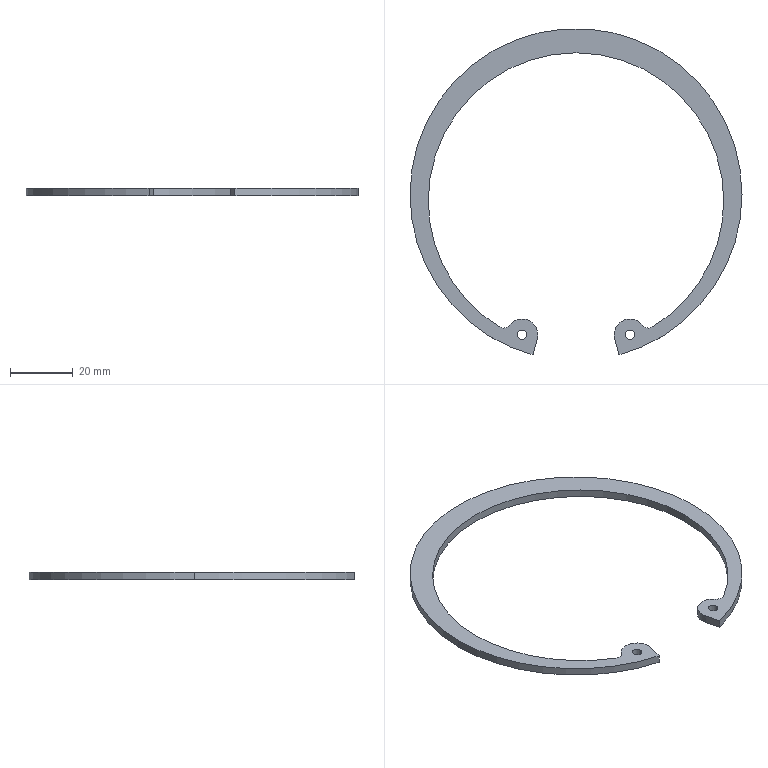Part | SolidWorks | features Extrusion 1 | 1 solid | 19 faces | box 105.5 x 103.703 x 2.5 mm | volume 4495 mm3 | cylinder 15 | plane 4 | commonest cylinder face diameters 3 x4 10 x3 93.9 x3 105.5 x3 5 x2
STEP:
#1=CARTESIAN_POINT('',(-18.607,-44.527,-2.5));
#2=VERTEX_POINT('',#1);
#3=CARTESIAN_POINT('',(-15.607,-44.527,-2.5));
#4=VERTEX_POINT('',#3);
#5=CARTESIAN_POINT('',(-17.107,-44.527,-2.5));
#6=DIRECTION('',(0.,0.,1.));
#7=DIRECTION('',(1.,0.,0.));
#8=AXIS2_PLACEMENT_3D('',#5,#6,#7);
#9=CIRCLE('',#8,1.5);
#10=EDGE_CURVE('',#2,#4,#9,.T.);
#11=ORIENTED_EDGE('',*,*,#10,.F.);
#12=CARTESIAN_POINT('',(-18.607,-44.527,0.));
#13=VERTEX_POINT('',#12);
#14=CARTESIAN_POINT('',(-18.607,-44.527,-2.5));
#15=DIRECTION('',(0.,0.,1.));
#16=VECTOR('',#15,1000.);
#17=LINE('',#14,#16);
#18=EDGE_CURVE('',#2,#13,#17,.T.);
#19=ORIENTED_EDGE('',*,*,#18,.T.);
#20=CARTESIAN_POINT('',(-15.607,-44.527,0.));
#21=VERTEX_POINT('',#20);
#22=CARTESIAN_POINT('',(-17.107,-44.527,0.));
#23=DIRECTION('',(0.,0.,1.));
#24=DIRECTION('',(1.,0.,0.));
#25=AXIS2_PLACEMENT_3D('',#22,#23,#24);
#26=CIRCLE('',#25,1.5);
#27=EDGE_CURVE('',#13,#21,#26,.T.);
#28=ORIENTED_EDGE('',*,*,#27,.T.);
#29=CARTESIAN_POINT('',(-15.607,-44.527,-2.5));
#30=DIRECTION('',(0.,0.,1.));
#31=VECTOR('',#30,1000.);
#32=LINE('',#29,#31);
#33=EDGE_CURVE('',#4,#21,#32,.T.);
#34=ORIENTED_EDGE('',*,*,#33,.F.);
#35=EDGE_LOOP('',(#11,#19,#28,#34));
#36=FACE_OUTER_BOUND('',#35,.T.);
#37=CARTESIAN_POINT('',(-17.107,-44.527,-2.5));
#38=DIRECTION('',(0.,0.,1.));
#39=DIRECTION('',(1.,0.,0.));
#40=AXIS2_PLACEMENT_3D('',#37,#38,#39);
#41=CYLINDRICAL_SURFACE('',#40,1.5);
#42=ADVANCED_FACE('',(#36),#41,.F.);
#43=CARTESIAN_POINT('',(15.607,-44.527,-2.5));
#44=VERTEX_POINT('',#43);
#45=CARTESIAN_POINT('',(18.607,-44.527,-2.5));
#46=VERTEX_POINT('',#45);
#47=CARTESIAN_POINT('',(17.107,-44.527,-2.5));
#48=DIRECTION('',(0.,0.,1.));
#49=DIRECTION('',(-1.,0.,0.));
#50=AXIS2_PLACEMENT_3D('',#47,#48,#49);
#51=CIRCLE('',#50,1.5);
#52=EDGE_CURVE('',#44,#46,#51,.T.);
#53=ORIENTED_EDGE('',*,*,#52,.F.);
#54=CARTESIAN_POINT('',(15.607,-44.527,0.));
#55=VERTEX_POINT('',#54);
#56=CARTESIAN_POINT('',(15.607,-44.527,-2.5));
#57=DIRECTION('',(0.,0.,1.));
#58=VECTOR('',#57,1000.);
#59=LINE('',#56,#58);
#60=EDGE_CURVE('',#44,#55,#59,.T.);
#61=ORIENTED_EDGE('',*,*,#60,.T.);
#62=CARTESIAN_POINT('',(18.607,-44.527,0.));
#63=VERTEX_POINT('',#62);
#64=CARTESIAN_POINT('',(17.107,-44.527,0.));
#65=DIRECTION('',(0.,0.,1.));
#66=DIRECTION('',(-1.,0.,0.));
#67=AXIS2_PLACEMENT_3D('',#64,#65,#66);
#68=CIRCLE('',#67,1.5);
#69=EDGE_CURVE('',#55,#63,#68,.T.);
#70=ORIENTED_EDGE('',*,*,#69,.T.);
#71=CARTESIAN_POINT('',(18.607,-44.527,-2.5));
#72=DIRECTION('',(0.,0.,1.));
#73=VECTOR('',#72,1000.);
#74=LINE('',#71,#73);
#75=EDGE_CURVE('',#46,#63,#74,.T.);
#76=ORIENTED_EDGE('',*,*,#75,.F.);
#77=EDGE_LOOP('',(#53,#61,#70,#76));
#78=FACE_OUTER_BOUND('',#77,.T.);
#79=CARTESIAN_POINT('',(17.107,-44.527,-2.5));
#80=DIRECTION('',(0.,0.,1.));
#81=DIRECTION('',(1.,0.,0.));
#82=AXIS2_PLACEMENT_3D('',#79,#80,#81);
#83=CYLINDRICAL_SURFACE('',#82,1.5);
#84=ADVANCED_FACE('',(#78),#83,.F.);
#85=CARTESIAN_POINT('',(-12.278,-45.821,-2.5));
#86=VERTEX_POINT('',#85);
#87=CARTESIAN_POINT('',(-12.107,-44.527,-2.5));
#88=VERTEX_POINT('',#87);
#89=CARTESIAN_POINT('',(-17.107,-44.527,-2.5));
#90=DIRECTION('',(0.,0.,1.));
#91=DIRECTION('',(1.,0.,0.));
#92=AXIS2_PLACEMENT_3D('',#89,#90,#91);
#93=CIRCLE('',#92,5.);
#94=EDGE_CURVE('',#86,#88,#93,.T.);
#95=ORIENTED_EDGE('',*,*,#94,.T.);
#96=CARTESIAN_POINT('',(-12.107,-44.527,0.));
#97=VERTEX_POINT('',#96);
#98=CARTESIAN_POINT('',(-12.107,-44.527,-2.5));
#99=DIRECTION('',(0.,0.,1.));
#100=VECTOR('',#99,1000.);
#101=LINE('',#98,#100);
#102=EDGE_CURVE('',#88,#97,#101,.T.);
#103=ORIENTED_EDGE('',*,*,#102,.T.);
#104=CARTESIAN_POINT('',(-12.278,-45.821,0.));
#105=VERTEX_POINT('',#104);
#106=CARTESIAN_POINT('',(-17.107,-44.527,0.));
#107=DIRECTION('',(0.,0.,1.));
#108=DIRECTION('',(1.,0.,0.));
#109=AXIS2_PLACEMENT_3D('',#106,#107,#108);
#110=CIRCLE('',#109,5.);
#111=EDGE_CURVE('',#105,#97,#110,.T.);
#112=ORIENTED_EDGE('',*,*,#111,.F.);
#113=CARTESIAN_POINT('',(-12.278,-45.821,-2.5));
#114=DIRECTION('',(0.,0.,1.));
#115=VECTOR('',#114,1000.);
#116=LINE('',#113,#115);
#117=EDGE_CURVE('',#86,#105,#116,.T.);
#118=ORIENTED_EDGE('',*,*,#117,.F.);
#119=EDGE_LOOP('',(#95,#103,#112,#118));
#120=FACE_OUTER_BOUND('',#119,.T.);
#121=CARTESIAN_POINT('',(-17.107,-44.527,-2.5));
#122=DIRECTION('',(0.,0.,1.));
#123=DIRECTION('',(1.,0.,0.));
#124=AXIS2_PLACEMENT_3D('',#121,#122,#123);
#125=CYLINDRICAL_SURFACE('',#124,5.);
#126=ADVANCED_FACE('',(#120),#125,.T.);
#127=CARTESIAN_POINT('',(-24.321,-42.059,-2.5));
#128=VERTEX_POINT('',#127);
#129=CARTESIAN_POINT('',(-46.95,-1.9,-2.5));
#130=VERTEX_POINT('',#129);
#131=CARTESIAN_POINT('',(0.,-1.9,-2.5));
#132=DIRECTION('',(0.,0.,-1.));
#133=DIRECTION('',(1.,0.,0.));
#134=AXIS2_PLACEMENT_3D('',#131,#132,#133);
#135=CIRCLE('',#134,46.95);
#136=EDGE_CURVE('',#128,#130,#135,.T.);
#137=ORIENTED_EDGE('',*,*,#136,.T.);
#138=CARTESIAN_POINT('',(-46.95,-1.9,0.));
#139=VERTEX_POINT('',#138);
#140=CARTESIAN_POINT('',(-46.95,-1.9,-2.5));
#141=DIRECTION('',(0.,0.,1.));
#142=VECTOR('',#141,1000.);
#143=LINE('',#140,#142);
#144=EDGE_CURVE('',#130,#139,#143,.T.);
#145=ORIENTED_EDGE('',*,*,#144,.T.);
#146=CARTESIAN_POINT('',(-24.321,-42.059,0.));
#147=VERTEX_POINT('',#146);
#148=CARTESIAN_POINT('',(0.,-1.9,0.));
#149=DIRECTION('',(0.,0.,-1.));
#150=DIRECTION('',(1.,0.,0.));
#151=AXIS2_PLACEMENT_3D('',#148,#149,#150);
#152=CIRCLE('',#151,46.95);
#153=EDGE_CURVE('',#147,#139,#152,.T.);
#154=ORIENTED_EDGE('',*,*,#153,.F.);
#155=CARTESIAN_POINT('',(-24.321,-42.059,-2.5));
#156=DIRECTION('',(0.,0.,1.));
#157=VECTOR('',#156,1000.);
#158=LINE('',#155,#157);
#159=EDGE_CURVE('',#128,#147,#158,.T.);
#160=ORIENTED_EDGE('',*,*,#159,.F.);
#161=EDGE_LOOP('',(#137,#145,#154,#160));
#162=FACE_OUTER_BOUND('',#161,.T.);
#163=CARTESIAN_POINT('',(0.,-1.9,-2.5));
#164=DIRECTION('',(0.,0.,1.));
#165=DIRECTION('',(1.,0.,0.));
#166=AXIS2_PLACEMENT_3D('',#163,#164,#165);
#167=CYLINDRICAL_SURFACE('',#166,46.95);
#168=ADVANCED_FACE('',(#162),#167,.F.);
#169=ORIENTED_EDGE('',*,*,#144,.F.);
#170=CARTESIAN_POINT('',(46.95,-1.9,-2.5));
#171=VERTEX_POINT('',#170);
#172=CARTESIAN_POINT('',(0.,-1.9,-2.5));
#173=DIRECTION('',(0.,0.,-1.));
#174=DIRECTION('',(1.,0.,0.));
#175=AXIS2_PLACEMENT_3D('',#172,#173,#174);
#176=CIRCLE('',#175,46.95);
#177=EDGE_CURVE('',#130,#171,#176,.T.);
#178=ORIENTED_EDGE('',*,*,#177,.T.);
#179=CARTESIAN_POINT('',(46.95,-1.9,0.));
#180=VERTEX_POINT('',#179);
#181=CARTESIAN_POINT('',(46.95,-1.9,-2.5));
#182=DIRECTION('',(0.,0.,1.));
#183=VECTOR('',#182,1000.);
#184=LINE('',#181,#183);
#185=EDGE_CURVE('',#171,#180,#184,.T.);
#186=ORIENTED_EDGE('',*,*,#185,.T.);
#187=CARTESIAN_POINT('',(0.,-1.9,0.));
#188=DIRECTION('',(0.,0.,-1.));
#189=DIRECTION('',(1.,0.,0.));
#190=AXIS2_PLACEMENT_3D('',#187,#188,#189);
#191=CIRCLE('',#190,46.95);
#192=EDGE_CURVE('',#139,#180,#191,.T.);
#193=ORIENTED_EDGE('',*,*,#192,.F.);
#194=EDGE_LOOP('',(#169,#178,#186,#193));
#195=FACE_OUTER_BOUND('',#194,.T.);
#196=CARTESIAN_POINT('',(0.,-1.9,-2.5));
#197=DIRECTION('',(0.,0.,1.));
#198=DIRECTION('',(1.,0.,0.));
#199=AXIS2_PLACEMENT_3D('',#196,#197,#198);
#200=CYLINDRICAL_SURFACE('',#199,46.95);
#201=ADVANCED_FACE('',(#195),#200,.F.);
#202=CARTESIAN_POINT('',(52.75,0.,-2.5));
#203=VERTEX_POINT('',#202);
#204=CARTESIAN_POINT('',(-52.75,0.,-2.5));
#205=VERTEX_POINT('',#204);
#206=CARTESIAN_POINT('',(0.,0.,-2.5));
#207=DIRECTION('',(0.,0.,1.));
#208=DIRECTION('',(1.,0.,0.));
#209=AXIS2_PLACEMENT_3D('',#206,#207,#208);
#210=CIRCLE('',#209,52.75);
#211=EDGE_CURVE('',#203,#205,#210,.T.);
#212=ORIENTED_EDGE('',*,*,#211,.T.);
#213=CARTESIAN_POINT('',(-52.75,0.,0.));
#214=VERTEX_POINT('',#213);
#215=CARTESIAN_POINT('',(-52.75,0.,-2.5));
#216=DIRECTION('',(0.,0.,1.));
#217=VECTOR('',#216,1000.);
#218=LINE('',#215,#217);
#219=EDGE_CURVE('',#205,#214,#218,.T.);
#220=ORIENTED_EDGE('',*,*,#219,.T.);
#221=CARTESIAN_POINT('',(52.75,0.,0.));
#222=VERTEX_POINT('',#221);
#223=CARTESIAN_POINT('',(0.,0.,0.));
#224=DIRECTION('',(0.,0.,1.));
#225=DIRECTION('',(1.,0.,0.));
#226=AXIS2_PLACEMENT_3D('',#223,#224,#225);
#227=CIRCLE('',#226,52.75);
#228=EDGE_CURVE('',#222,#214,#227,.T.);
#229=ORIENTED_EDGE('',*,*,#228,.F.);
#230=CARTESIAN_POINT('',(52.75,0.,-2.5));
#231=DIRECTION('',(0.,0.,1.));
#232=VECTOR('',#231,1000.);
#233=LINE('',#230,#232);
#234=EDGE_CURVE('',#203,#222,#233,.T.);
#235=ORIENTED_EDGE('',*,*,#234,.F.);
#236=EDGE_LOOP('',(#212,#220,#229,#235));
#237=FACE_OUTER_BOUND('',#236,.T.);
#238=CARTESIAN_POINT('',(0.,0.,-2.5));
#239=DIRECTION('',(0.,0.,1.));
#240=DIRECTION('',(1.,0.,0.));
#241=AXIS2_PLACEMENT_3D('',#238,#239,#240);
#242=CYLINDRICAL_SURFACE('',#241,52.75);
#243=ADVANCED_FACE('',(#237),#242,.T.);
#244=CARTESIAN_POINT('',(13.653,-50.953,-2.5));
#245=VERTEX_POINT('',#244);
#246=CARTESIAN_POINT('',(0.,0.,-2.5));
#247=DIRECTION('',(0.,0.,1.));
#248=DIRECTION('',(1.,0.,0.));
#249=AXIS2_PLACEMENT_3D('',#246,#247,#248);
#250=CIRCLE('',#249,52.75);
#251=EDGE_CURVE('',#245,#203,#250,.T.);
#252=ORIENTED_EDGE('',*,*,#251,.T.);
#253=ORIENTED_EDGE('',*,*,#234,.T.);
#254=CARTESIAN_POINT('',(13.653,-50.953,0.));
#255=VERTEX_POINT('',#254);
#256=CARTESIAN_POINT('',(0.,0.,0.));
#257=DIRECTION('',(0.,0.,1.));
#258=DIRECTION('',(1.,0.,0.));
#259=AXIS2_PLACEMENT_3D('',#256,#257,#258);
#260=CIRCLE('',#259,52.75);
#261=EDGE_CURVE('',#255,#222,#260,.T.);
#262=ORIENTED_EDGE('',*,*,#261,.F.);
#263=CARTESIAN_POINT('',(13.653,-50.953,-2.5));
#264=DIRECTION('',(0.,0.,1.));
#265=VECTOR('',#264,1000.);
#266=LINE('',#263,#265);
#267=EDGE_CURVE('',#245,#255,#266,.T.);
#268=ORIENTED_EDGE('',*,*,#267,.F.);
#269=EDGE_LOOP('',(#252,#253,#262,#268));
#270=FACE_OUTER_BOUND('',#269,.T.);
#271=CARTESIAN_POINT('',(0.,0.,-2.5));
#272=DIRECTION('',(0.,0.,1.));
#273=DIRECTION('',(1.,0.,0.));
#274=AXIS2_PLACEMENT_3D('',#271,#272,#273);
#275=CYLINDRICAL_SURFACE('',#274,52.75);
#276=ADVANCED_FACE('',(#270),#275,.T.);
#277=ORIENTED_EDGE('',*,*,#219,.F.);
#278=CARTESIAN_POINT('',(-13.653,-50.953,-2.5));
#279=VERTEX_POINT('',#278);
#280=CARTESIAN_POINT('',(0.,0.,-2.5));
#281=DIRECTION('',(0.,0.,1.));
#282=DIRECTION('',(1.,0.,0.));
#283=AXIS2_PLACEMENT_3D('',#280,#281,#282);
#284=CIRCLE('',#283,52.75);
#285=EDGE_CURVE('',#205,#279,#284,.T.);
#286=ORIENTED_EDGE('',*,*,#285,.T.);
#287=CARTESIAN_POINT('',(-13.653,-50.953,0.));
#288=VERTEX_POINT('',#287);
#289=CARTESIAN_POINT('',(-13.653,-50.953,-2.5));
#290=DIRECTION('',(0.,0.,1.));
#291=VECTOR('',#290,1000.);
#292=LINE('',#289,#291);
#293=EDGE_CURVE('',#279,#288,#292,.T.);
#294=ORIENTED_EDGE('',*,*,#293,.T.);
#295=CARTESIAN_POINT('',(0.,0.,0.));
#296=DIRECTION('',(0.,0.,1.));
#297=DIRECTION('',(1.,0.,0.));
#298=AXIS2_PLACEMENT_3D('',#295,#296,#297);
#299=CIRCLE('',#298,52.75);
#300=EDGE_CURVE('',#214,#288,#299,.T.);
#301=ORIENTED_EDGE('',*,*,#300,.F.);
#302=EDGE_LOOP('',(#277,#286,#294,#301));
#303=FACE_OUTER_BOUND('',#302,.T.);
#304=CARTESIAN_POINT('',(0.,0.,-2.5));
#305=DIRECTION('',(0.,0.,1.));
#306=DIRECTION('',(1.,0.,0.));
#307=AXIS2_PLACEMENT_3D('',#304,#305,#306);
#308=CYLINDRICAL_SURFACE('',#307,52.75);
#309=ADVANCED_FACE('',(#303),#308,.T.);
#310=CARTESIAN_POINT('',(12.278,-45.821,0.));
#311=VERTEX_POINT('',#310);
#312=CARTESIAN_POINT('',(12.278,-45.821,0.));
#313=DIRECTION('',(0.2588,-0.9659,0.));
#314=VECTOR('',#313,1000.);
#315=LINE('',#312,#314);
#316=EDGE_CURVE('',#311,#255,#315,.T.);
#317=ORIENTED_EDGE('',*,*,#316,.F.);
#318=CARTESIAN_POINT('',(12.278,-45.821,-2.5));
#319=VERTEX_POINT('',#318);
#320=CARTESIAN_POINT('',(12.278,-45.821,-2.5));
#321=DIRECTION('',(0.,0.,1.));
#322=VECTOR('',#321,1000.);
#323=LINE('',#320,#322);
#324=EDGE_CURVE('',#319,#311,#323,.T.);
#325=ORIENTED_EDGE('',*,*,#324,.F.);
#326=CARTESIAN_POINT('',(12.278,-45.821,-2.5));
#327=DIRECTION('',(0.2588,-0.9659,0.));
#328=VECTOR('',#327,1000.);
#329=LINE('',#326,#328);
#330=EDGE_CURVE('',#319,#245,#329,.T.);
#331=ORIENTED_EDGE('',*,*,#330,.T.);
#332=ORIENTED_EDGE('',*,*,#267,.T.);
#333=EDGE_LOOP('',(#317,#325,#331,#332));
#334=FACE_OUTER_BOUND('',#333,.T.);
#335=CARTESIAN_POINT('',(12.278,-45.821,-2.5));
#336=DIRECTION('',(-0.9659,-0.2588,0.));
#337=DIRECTION('',(0.2588,-0.9659,0.));
#338=AXIS2_PLACEMENT_3D('',#335,#336,#337);
#339=PLANE('',#338);
#340=ADVANCED_FACE('',(#334),#339,.T.);
#341=CARTESIAN_POINT('',(21.053,-41.456,0.));
#342=VERTEX_POINT('',#341);
#343=CARTESIAN_POINT('',(17.107,-44.527,0.));
#344=DIRECTION('',(0.,0.,1.));
#345=DIRECTION('',(-1.,0.,0.));
#346=AXIS2_PLACEMENT_3D('',#343,#344,#345);
#347=CIRCLE('',#346,5.);
#348=EDGE_CURVE('',#342,#311,#347,.T.);
#349=ORIENTED_EDGE('',*,*,#348,.F.);
#350=CARTESIAN_POINT('',(21.053,-41.456,-2.5));
#351=VERTEX_POINT('',#350);
#352=CARTESIAN_POINT('',(21.053,-41.456,-2.5));
#353=DIRECTION('',(0.,0.,1.));
#354=VECTOR('',#353,1000.);
#355=LINE('',#352,#354);
#356=EDGE_CURVE('',#351,#342,#355,.T.);
#357=ORIENTED_EDGE('',*,*,#356,.F.);
#358=CARTESIAN_POINT('',(17.107,-44.527,-2.5));
#359=DIRECTION('',(0.,0.,1.));
#360=DIRECTION('',(-1.,0.,0.));
#361=AXIS2_PLACEMENT_3D('',#358,#359,#360);
#362=CIRCLE('',#361,5.);
#363=EDGE_CURVE('',#351,#319,#362,.T.);
#364=ORIENTED_EDGE('',*,*,#363,.T.);
#365=ORIENTED_EDGE('',*,*,#324,.T.);
#366=EDGE_LOOP('',(#349,#357,#364,#365));
#367=FACE_OUTER_BOUND('',#366,.T.);
#368=CARTESIAN_POINT('',(17.107,-44.527,-2.5));
#369=DIRECTION('',(0.,0.,1.));
#370=DIRECTION('',(1.,0.,0.));
#371=AXIS2_PLACEMENT_3D('',#368,#369,#370);
#372=CYLINDRICAL_SURFACE('',#371,5.);
#373=ADVANCED_FACE('',(#367),#372,.T.);
#374=CARTESIAN_POINT('',(24.321,-42.059,0.));
#375=VERTEX_POINT('',#374);
#376=CARTESIAN_POINT('',(23.026,-39.921,0.));
#377=DIRECTION('',(0.,0.,-1.));
#378=DIRECTION('',(-1.,0.,0.));
#379=AXIS2_PLACEMENT_3D('',#376,#377,#378);
#380=CIRCLE('',#379,2.5);
#381=EDGE_CURVE('',#375,#342,#380,.T.);
#382=ORIENTED_EDGE('',*,*,#381,.F.);
#383=CARTESIAN_POINT('',(24.321,-42.059,-2.5));
#384=VERTEX_POINT('',#383);
#385=CARTESIAN_POINT('',(24.321,-42.059,-2.5));
#386=DIRECTION('',(0.,0.,1.));
#387=VECTOR('',#386,1000.);
#388=LINE('',#385,#387);
#389=EDGE_CURVE('',#384,#375,#388,.T.);
#390=ORIENTED_EDGE('',*,*,#389,.F.);
#391=CARTESIAN_POINT('',(23.026,-39.921,-2.5));
#392=DIRECTION('',(0.,0.,-1.));
#393=DIRECTION('',(-1.,0.,0.));
#394=AXIS2_PLACEMENT_3D('',#391,#392,#393);
#395=CIRCLE('',#394,2.5);
#396=EDGE_CURVE('',#384,#351,#395,.T.);
#397=ORIENTED_EDGE('',*,*,#396,.T.);
#398=ORIENTED_EDGE('',*,*,#356,.T.);
#399=EDGE_LOOP('',(#382,#390,#397,#398));
#400=FACE_OUTER_BOUND('',#399,.T.);
#401=CARTESIAN_POINT('',(23.026,-39.921,-2.5));
#402=DIRECTION('',(0.,0.,1.));
#403=DIRECTION('',(1.,0.,0.));
#404=AXIS2_PLACEMENT_3D('',#401,#402,#403);
#405=CYLINDRICAL_SURFACE('',#404,2.5);
#406=ADVANCED_FACE('',(#400),#405,.F.);
#407=ORIENTED_EDGE('',*,*,#185,.F.);
#408=CARTESIAN_POINT('',(0.,-1.9,-2.5));
#409=DIRECTION('',(0.,0.,-1.));
#410=DIRECTION('',(1.,0.,0.));
#411=AXIS2_PLACEMENT_3D('',#408,#409,#410);
#412=CIRCLE('',#411,46.95);
#413=EDGE_CURVE('',#171,#384,#412,.T.);
#414=ORIENTED_EDGE('',*,*,#413,.T.);
#415=ORIENTED_EDGE('',*,*,#389,.T.);
#416=CARTESIAN_POINT('',(0.,-1.9,0.));
#417=DIRECTION('',(0.,0.,-1.));
#418=DIRECTION('',(1.,0.,0.));
#419=AXIS2_PLACEMENT_3D('',#416,#417,#418);
#420=CIRCLE('',#419,46.95);
#421=EDGE_CURVE('',#180,#375,#420,.T.);
#422=ORIENTED_EDGE('',*,*,#421,.F.);
#423=EDGE_LOOP('',(#407,#414,#415,#422));
#424=FACE_OUTER_BOUND('',#423,.T.);
#425=CARTESIAN_POINT('',(0.,-1.9,-2.5));
#426=DIRECTION('',(0.,0.,1.));
#427=DIRECTION('',(1.,0.,0.));
#428=AXIS2_PLACEMENT_3D('',#425,#426,#427);
#429=CYLINDRICAL_SURFACE('',#428,46.95);
#430=ADVANCED_FACE('',(#424),#429,.F.);
#431=CARTESIAN_POINT('',(-21.053,-41.456,0.));
#432=VERTEX_POINT('',#431);
#433=CARTESIAN_POINT('',(-23.026,-39.921,0.));
#434=DIRECTION('',(0.,0.,-1.));
#435=DIRECTION('',(1.,0.,0.));
#436=AXIS2_PLACEMENT_3D('',#433,#434,#435);
#437=CIRCLE('',#436,2.5);
#438=EDGE_CURVE('',#432,#147,#437,.T.);
#439=ORIENTED_EDGE('',*,*,#438,.F.);
#440=CARTESIAN_POINT('',(-21.053,-41.456,-2.5));
#441=VERTEX_POINT('',#440);
#442=CARTESIAN_POINT('',(-21.053,-41.456,-2.5));
#443=DIRECTION('',(0.,0.,1.));
#444=VECTOR('',#443,1000.);
#445=LINE('',#442,#444);
#446=EDGE_CURVE('',#441,#432,#445,.T.);
#447=ORIENTED_EDGE('',*,*,#446,.F.);
#448=CARTESIAN_POINT('',(-23.026,-39.921,-2.5));
#449=DIRECTION('',(0.,0.,-1.));
#450=DIRECTION('',(1.,0.,0.));
#451=AXIS2_PLACEMENT_3D('',#448,#449,#450);
#452=CIRCLE('',#451,2.5);
#453=EDGE_CURVE('',#441,#128,#452,.T.);
#454=ORIENTED_EDGE('',*,*,#453,.T.);
#455=ORIENTED_EDGE('',*,*,#159,.T.);
#456=EDGE_LOOP('',(#439,#447,#454,#455));
#457=FACE_OUTER_BOUND('',#456,.T.);
#458=CARTESIAN_POINT('',(-23.026,-39.921,-2.5));
#459=DIRECTION('',(0.,0.,1.));
#460=DIRECTION('',(1.,0.,0.));
#461=AXIS2_PLACEMENT_3D('',#458,#459,#460);
#462=CYLINDRICAL_SURFACE('',#461,2.5);
#463=ADVANCED_FACE('',(#457),#462,.F.);
#464=ORIENTED_EDGE('',*,*,#102,.F.);
#465=CARTESIAN_POINT('',(-17.107,-44.527,-2.5));
#466=DIRECTION('',(0.,0.,1.));
#467=DIRECTION('',(1.,0.,0.));
#468=AXIS2_PLACEMENT_3D('',#465,#466,#467);
#469=CIRCLE('',#468,5.);
#470=EDGE_CURVE('',#88,#441,#469,.T.);
#471=ORIENTED_EDGE('',*,*,#470,.T.);
#472=ORIENTED_EDGE('',*,*,#446,.T.);
#473=CARTESIAN_POINT('',(-17.107,-44.527,0.));
#474=DIRECTION('',(0.,0.,1.));
#475=DIRECTION('',(1.,0.,0.));
#476=AXIS2_PLACEMENT_3D('',#473,#474,#475);
#477=CIRCLE('',#476,5.);
#478=EDGE_CURVE('',#97,#432,#477,.T.);
#479=ORIENTED_EDGE('',*,*,#478,.F.);
#480=EDGE_LOOP('',(#464,#471,#472,#479));
#481=FACE_OUTER_BOUND('',#480,.T.);
#482=CARTESIAN_POINT('',(-17.107,-44.527,-2.5));
#483=DIRECTION('',(0.,0.,1.));
#484=DIRECTION('',(1.,0.,0.));
#485=AXIS2_PLACEMENT_3D('',#482,#483,#484);
#486=CYLINDRICAL_SURFACE('',#485,5.);
#487=ADVANCED_FACE('',(#481),#486,.T.);
#488=CARTESIAN_POINT('',(-12.278,-45.821,0.));
#489=DIRECTION('',(0.2588,0.9659,0.));
#490=VECTOR('',#489,1000.);
#491=LINE('',#488,#490);
#492=EDGE_CURVE('',#288,#105,#491,.T.);
#493=ORIENTED_EDGE('',*,*,#492,.F.);
#494=ORIENTED_EDGE('',*,*,#293,.F.);
#495=CARTESIAN_POINT('',(-12.278,-45.821,-2.5));
#496=DIRECTION('',(0.2588,0.9659,0.));
#497=VECTOR('',#496,1000.);
#498=LINE('',#495,#497);
#499=EDGE_CURVE('',#279,#86,#498,.T.);
#500=ORIENTED_EDGE('',*,*,#499,.T.);
#501=ORIENTED_EDGE('',*,*,#117,.T.);
#502=EDGE_LOOP('',(#493,#494,#500,#501));
#503=FACE_OUTER_BOUND('',#502,.T.);
#504=CARTESIAN_POINT('',(-12.278,-45.821,-2.5));
#505=DIRECTION('',(0.9659,-0.2588,0.));
#506=DIRECTION('',(0.2588,0.9659,0.));
#507=AXIS2_PLACEMENT_3D('',#504,#505,#506);
#508=PLANE('',#507);
#509=ADVANCED_FACE('',(#503),#508,.T.);
#510=CARTESIAN_POINT('',(-17.107,-44.527,-2.5));
#511=DIRECTION('',(0.,0.,1.));
#512=DIRECTION('',(1.,0.,0.));
#513=AXIS2_PLACEMENT_3D('',#510,#511,#512);
#514=CIRCLE('',#513,1.5);
#515=EDGE_CURVE('',#4,#2,#514,.T.);
#516=ORIENTED_EDGE('',*,*,#515,.T.);
#517=ORIENTED_EDGE('',*,*,#10,.T.);
#518=EDGE_LOOP('',(#516,#517));
#519=FACE_BOUND('',#518,.T.);
#520=CARTESIAN_POINT('',(17.107,-44.527,-2.5));
#521=DIRECTION('',(0.,0.,1.));
#522=DIRECTION('',(-1.,0.,0.));
#523=AXIS2_PLACEMENT_3D('',#520,#521,#522);
#524=CIRCLE('',#523,1.5);
#525=EDGE_CURVE('',#46,#44,#524,.T.);
#526=ORIENTED_EDGE('',*,*,#525,.T.);
#527=ORIENTED_EDGE('',*,*,#52,.T.);
#528=EDGE_LOOP('',(#526,#527));
#529=FACE_BOUND('',#528,.T.);
#530=ORIENTED_EDGE('',*,*,#251,.F.);
#531=ORIENTED_EDGE('',*,*,#330,.F.);
#532=ORIENTED_EDGE('',*,*,#363,.F.);
#533=ORIENTED_EDGE('',*,*,#396,.F.);
#534=ORIENTED_EDGE('',*,*,#413,.F.);
#535=ORIENTED_EDGE('',*,*,#177,.F.);
#536=ORIENTED_EDGE('',*,*,#136,.F.);
#537=ORIENTED_EDGE('',*,*,#453,.F.);
#538=ORIENTED_EDGE('',*,*,#470,.F.);
#539=ORIENTED_EDGE('',*,*,#94,.F.);
#540=ORIENTED_EDGE('',*,*,#499,.F.);
#541=ORIENTED_EDGE('',*,*,#285,.F.);
#542=ORIENTED_EDGE('',*,*,#211,.F.);
#543=EDGE_LOOP('',(#530,#531,#532,#533,#534,#535,#536,#537,#538,#539,#540,#541,#542));
#544=FACE_OUTER_BOUND('',#543,.T.);
#545=CARTESIAN_POINT('',(0.,0.,-2.5));
#546=DIRECTION('',(0.,0.,1.));
#547=DIRECTION('',(1.,0.,0.));
#548=AXIS2_PLACEMENT_3D('',#545,#546,#547);
#549=PLANE('',#548);
#550=ADVANCED_FACE('',(#519,#529,#544),#549,.F.);
#551=CARTESIAN_POINT('',(-17.107,-44.527,0.));
#552=DIRECTION('',(0.,0.,1.));
#553=DIRECTION('',(1.,0.,0.));
#554=AXIS2_PLACEMENT_3D('',#551,#552,#553);
#555=CIRCLE('',#554,1.5);
#556=EDGE_CURVE('',#21,#13,#555,.T.);
#557=ORIENTED_EDGE('',*,*,#556,.F.);
#558=ORIENTED_EDGE('',*,*,#27,.F.);
#559=EDGE_LOOP('',(#557,#558));
#560=FACE_BOUND('',#559,.T.);
#561=CARTESIAN_POINT('',(17.107,-44.527,0.));
#562=DIRECTION('',(0.,0.,1.));
#563=DIRECTION('',(-1.,0.,0.));
#564=AXIS2_PLACEMENT_3D('',#561,#562,#563);
#565=CIRCLE('',#564,1.5);
#566=EDGE_CURVE('',#63,#55,#565,.T.);
#567=ORIENTED_EDGE('',*,*,#566,.F.);
#568=ORIENTED_EDGE('',*,*,#69,.F.);
#569=EDGE_LOOP('',(#567,#568));
#570=FACE_BOUND('',#569,.T.);
#571=ORIENTED_EDGE('',*,*,#261,.T.);
#572=ORIENTED_EDGE('',*,*,#228,.T.);
#573=ORIENTED_EDGE('',*,*,#300,.T.);
#574=ORIENTED_EDGE('',*,*,#492,.T.);
#575=ORIENTED_EDGE('',*,*,#111,.T.);
#576=ORIENTED_EDGE('',*,*,#478,.T.);
#577=ORIENTED_EDGE('',*,*,#438,.T.);
#578=ORIENTED_EDGE('',*,*,#153,.T.);
#579=ORIENTED_EDGE('',*,*,#192,.T.);
#580=ORIENTED_EDGE('',*,*,#421,.T.);
#581=ORIENTED_EDGE('',*,*,#381,.T.);
#582=ORIENTED_EDGE('',*,*,#348,.T.);
#583=ORIENTED_EDGE('',*,*,#316,.T.);
#584=EDGE_LOOP('',(#571,#572,#573,#574,#575,#576,#577,#578,#579,#580,#581,#582,#583));
#585=FACE_OUTER_BOUND('',#584,.T.);
#586=CARTESIAN_POINT('',(0.,0.,0.));
#587=DIRECTION('',(0.,0.,1.));
#588=DIRECTION('',(1.,0.,0.));
#589=AXIS2_PLACEMENT_3D('',#586,#587,#588);
#590=PLANE('',#589);
#591=ADVANCED_FACE('',(#560,#570,#585),#590,.T.);
#592=ORIENTED_EDGE('',*,*,#60,.F.);
#593=ORIENTED_EDGE('',*,*,#525,.F.);
#594=ORIENTED_EDGE('',*,*,#75,.T.);
#595=ORIENTED_EDGE('',*,*,#566,.T.);
#596=EDGE_LOOP('',(#592,#593,#594,#595));
#597=FACE_OUTER_BOUND('',#596,.T.);
#598=CARTESIAN_POINT('',(17.107,-44.527,-2.5));
#599=DIRECTION('',(0.,0.,1.));
#600=DIRECTION('',(1.,0.,0.));
#601=AXIS2_PLACEMENT_3D('',#598,#599,#600);
#602=CYLINDRICAL_SURFACE('',#601,1.5);
#603=ADVANCED_FACE('',(#597),#602,.F.);
#604=ORIENTED_EDGE('',*,*,#18,.F.);
#605=ORIENTED_EDGE('',*,*,#515,.F.);
#606=ORIENTED_EDGE('',*,*,#33,.T.);
#607=ORIENTED_EDGE('',*,*,#556,.T.);
#608=EDGE_LOOP('',(#604,#605,#606,#607));
#609=FACE_OUTER_BOUND('',#608,.T.);
#610=CARTESIAN_POINT('',(-17.107,-44.527,-2.5));
#611=DIRECTION('',(0.,0.,1.));
#612=DIRECTION('',(1.,0.,0.));
#613=AXIS2_PLACEMENT_3D('',#610,#611,#612);
#614=CYLINDRICAL_SURFACE('',#613,1.5);
#615=ADVANCED_FACE('',(#609),#614,.F.);
#616=CLOSED_SHELL('',(#42,#84,#126,#168,#201,#243,#276,#309,#340,#373,#406,#430,#463,#487,#509,#550,#591,#603,#615));
#617=MANIFOLD_SOLID_BREP('',#616);
#618=CARTESIAN_POINT('',(0.,0.,0.));
#619=DIRECTION('',(0.,0.,1.));
#620=DIRECTION('',(1.,0.,0.));
#621=AXIS2_PLACEMENT_3D('',#618,#619,#620);
#622=(LENGTH_UNIT()NAMED_UNIT(*)SI_UNIT(.MILLI.,.METRE.));
#623=UNCERTAINTY_MEASURE_WITH_UNIT(LENGTH_MEASURE(0.00001),#622,'','');
#624=(NAMED_UNIT(*)PLANE_ANGLE_UNIT()SI_UNIT($,.RADIAN.));
#625=(NAMED_UNIT(*)SI_UNIT($,.STERADIAN.)SOLID_ANGLE_UNIT());
#626=(GEOMETRIC_REPRESENTATION_CONTEXT(3)GLOBAL_UNCERTAINTY_ASSIGNED_CONTEXT((#623))GLOBAL_UNIT_ASSIGNED_CONTEXT((#622,#624,#625))REPRESENTATION_CONTEXT('',''));
#627=ADVANCED_BREP_SHAPE_REPRESENTATION('',(#617,#621),#626);